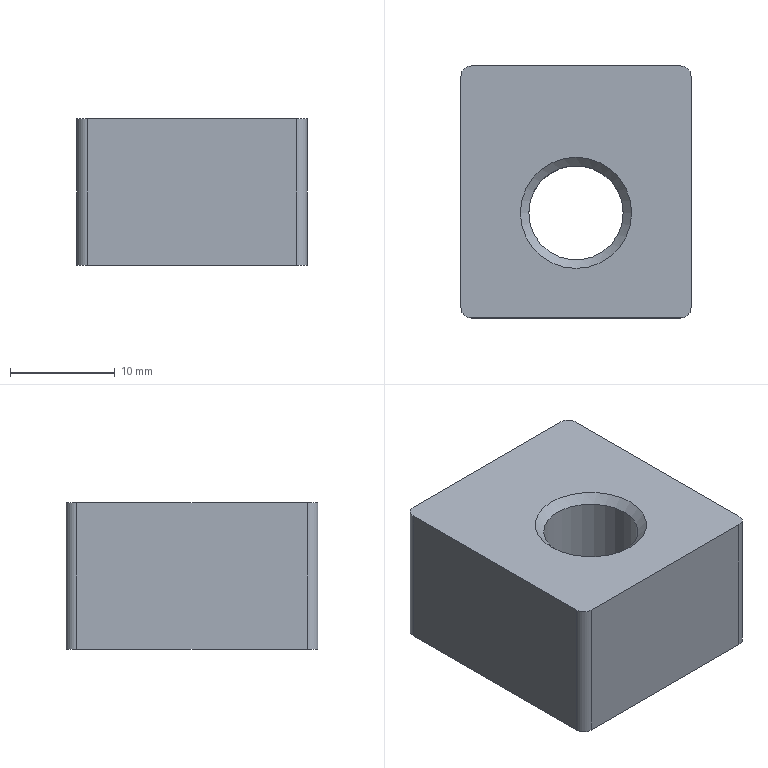NC program | NX | posted with a generic post | part box 21.95 x 24 x 14 mm
Whole program:
N10 G17 G21 G94 G90
(PLANAR_MILL_COPY_1_COPY_COPY , TOOL : D16CU)
N12 T01 M6
N14 G53
N16 G17 G0 G90 X-4. Y20.201 S2200 M3
N18 G43 Z56. H1
N20 Z5.7
N22 G94 G1 Y12.3 F1200.
N24 G3 X-2. Y10.3 R2.
N26 G2 X8.3 Y0. R10.3
N28 X-2. Y10.3 R-10.3
N30 G3 X0. Y12.3 R2.
N32 G1 Y20.201
N34 G0 X-4. Z5.4
N36 G1 Y12.3
N38 G3 X-2. Y10.3 R2.
N40 G2 X8.3 Y0. R10.3
N42 X-2. Y10.3 R-10.3
N44 G3 X0. Y12.3 R2.
N46 G1 Y20.201
N48 G0 X-4. Z5.1
N50 G1 Y12.3
N52 G3 X-2. Y10.3 R2.
N54 G2 X8.3 Y0. R10.3
N56 X-2. Y10.3 R-10.3
N58 G3 X0. Y12.3 R2.
N60 G1 Y20.201
N62 G0 X-4. Z4.8
N64 G1 Y12.3
N66 G3 X-2. Y10.3 R2.
N68 G2 X8.3 Y0. R10.3
N70 X-2. Y10.3 R-10.3
N72 G3 X0. Y12.3 R2.
N74 G1 Y20.201
N76 G0 X-4. Z4.5
N78 G1 Y12.3
N80 G3 X-2. Y10.3 R2.
N82 G2 X8.3 Y0. R10.3
N84 X-2. Y10.3 R-10.3
N86 G3 X0. Y12.3 R2.
N88 G1 Y20.201
N90 G0 X-4. Z4.2
N92 G1 Y12.3
N94 G3 X-2. Y10.3 R2.
N96 G2 X8.3 Y0. R10.3
N98 X-2. Y10.3 R-10.3
N100 G3 X0. Y12.3 R2.
N102 G1 Y20.201
N104 G0 X-4. Z3.9
N106 G1 Y12.3
N108 G3 X-2. Y10.3 R2.
N110 G2 X8.3 Y0. R10.3
N112 X-2. Y10.3 R-10.3
N114 G3 X0. Y12.3 R2.
N116 G1 Y20.201
N118 G0 X-4. Z3.6
N120 G1 Y12.3
N122 G3 X-2. Y10.3 R2.
N124 G2 X8.3 Y0. R10.3
N126 X-2. Y10.3 R-10.3
N128 G3 X0. Y12.3 R2.
N130 G1 Y20.201
N132 G0 X-4. Z3.3
N134 G1 Y12.3
N136 G3 X-2. Y10.3 R2.
N138 G2 X8.3 Y0. R10.3
N140 X-2. Y10.3 R-10.3
N142 G3 X0. Y12.3 R2.
N144 G1 Y20.201
N146 G0 X-4. Z3.
N148 G1 Y12.3
N150 G3 X-2. Y10.3 R2.
N152 G2 X8.3 Y0. R10.3
N154 X-2. Y10.3 R-10.3
N156 G3 X0. Y12.3 R2.
N158 G1 Y20.201
N160 G0 X-4. Z2.7
N162 G1 Y12.3
N164 G3 X-2. Y10.3 R2.
N166 G2 X8.3 Y0. R10.3
N168 X-2. Y10.3 R-10.3
N170 G3 X0. Y12.3 R2.
N172 G1 Y20.201
N174 G0 X-4. Z2.4
N176 G1 Y12.3
N178 G3 X-2. Y10.3 R2.
N180 G2 X8.3 Y0. R10.3
N182 X-2. Y10.3 R-10.3
N184 G3 X0. Y12.3 R2.
N186 G1 Y20.201
N188 G0 X-4. Z2.1
N190 G1 Y12.3
N192 G3 X-2. Y10.3 R2.
N194 G2 X8.3 Y0. R10.3
N196 X-2. Y10.3 R-10.3
N198 G3 X0. Y12.3 R2.
N200 G1 Y20.201
N202 G0 X-4. Z1.8
N204 G1 Y12.3
N206 G3 X-2. Y10.3 R2.
N208 G2 X8.3 Y0. R10.3
N210 X-2. Y10.3 R-10.3
N212 G3 X0. Y12.3 R2.
N214 G1 Y20.201
N216 G0 X-4. Z1.5
N218 G1 Y12.3
N220 G3 X-2. Y10.3 R2.
N222 G2 X8.3 Y0. R10.3
N224 X-2. Y10.3 R-10.3
N226 G3 X0. Y12.3 R2.
N228 G1 Y20.201
N230 G0 X-4. Z1.2
N232 G1 Y12.3
N234 G3 X-2. Y10.3 R2.
N236 G2 X8.3 Y0. R10.3
N238 X-2. Y10.3 R-10.3
N240 G3 X0. Y12.3 R2.
N242 G1 Y20.201
N244 G0 X-4. Z0.9
N246 G1 Y12.3
N248 G3 X-2. Y10.3 R2.
N250 G2 X8.3 Y0. R10.3
N252 X-2. Y10.3 R-10.3
N254 G3 X0. Y12.3 R2.
N256 G1 Y20.201
N258 G0 X-4. Z0.6
N260 G1 Y12.3
N262 G3 X-2. Y10.3 R2.
N264 G2 X8.3 Y0. R10.3
N266 X-2. Y10.3 R-10.3
N268 G3 X0. Y12.3 R2.
N270 G1 Y20.201
N272 G0 X-4. Z0.3
N274 G1 Y12.3
N276 G3 X-2. Y10.3 R2.
N278 G2 X8.3 Y0. R10.3
N280 X-2. Y10.3 R-10.3
N282 G3 X0. Y12.3 R2.
N284 G1 Y20.201
N286 G0 X-4. Z0.1
N288 G1 Y12.3
N290 G3 X-2. Y10.3 R2.
N292 G2 X8.3 Y0. R10.3
N294 X-2. Y10.3 R-10.3
N296 G3 X0. Y12.3 R2.
N298 G1 Y20.201
N300 G0 Z56.
N302 M5
(PLANAR_MILL_COPY_1_COPY_1 , TOOL : D16.)
N304 T02 M6
N306 G53
N308 G17 G0 G90 X-4. Y20.704 S1600 M3
N310 G43 Z50. H2
N312 Z0.
N314 G94 G1 Y12.8 F400.
N316 G3 X-2. Y10.8 R2.
N318 G2 X8.8 Y0. R10.8
N320 X-2. Y10.8 R-10.8
N322 G3 X0. Y12.8 R2.
N324 G1 Y20.704
N326 G0 Z50.
N328 M5
(PLANAR_MILL_COPY_COPY , TOOL : D8点钻)
N330 T03 M6
N332 G53
N334 G17 G0 G90 X-16.8 Y7.975 S4500 M3
N336 G43 Z50. H3
N338 Z-3.
N340 G94 G3 X-14.8 Y9.975 R2. F1200.
N342 G2 X-11. Y13.775 R3.8
N344 G1 X11.
N346 G2 X14.8 Y9.975 R3.8
N348 G1 Y-9.975
N350 G2 X11. Y-13.775 R3.8
N352 G1 X-11.
N354 G2 X-14.8 Y-9.975 R3.8
N356 G1 Y9.975
N358 G3 X-16.455 Y11.945 R2.
N360 G0 Z50.
(PLANAR_MILL_COPY_COPY_COPY , TOOL : D8点钻)
N362 X-1. Y0.831
N364 Z-3.
N366 G1 Y1.3
N368 G3 X-2. Y2.3 R1.
N370 X-4.3 Y0. R2.3
N372 X-2. Y2.3 R-2.3
N374 X-3. Y1.3 R1.
N376 G1 Y0.831
N378 G0 Z50.
N380 M5
N382 M2